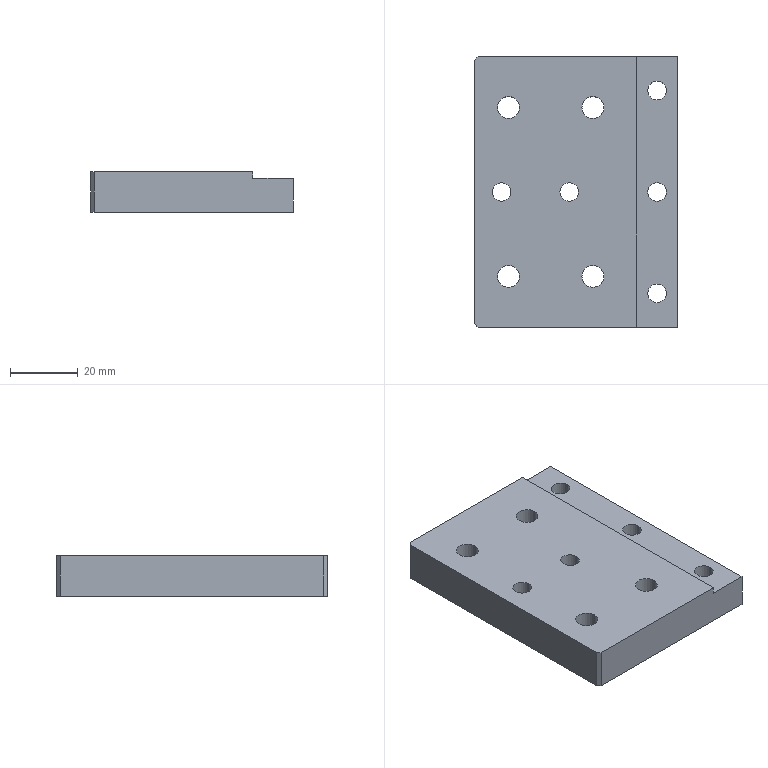Part | STEP file | PN_0044 Mount electronic clip mounting base plate B | 1 solid | 43 faces | box 60 x 80 x 12 mm | volume 51231 mm3 | cylinder 28 | plane 15 | commonest cylinder face diameters 5.5 x10 10 x10 6.5 x8